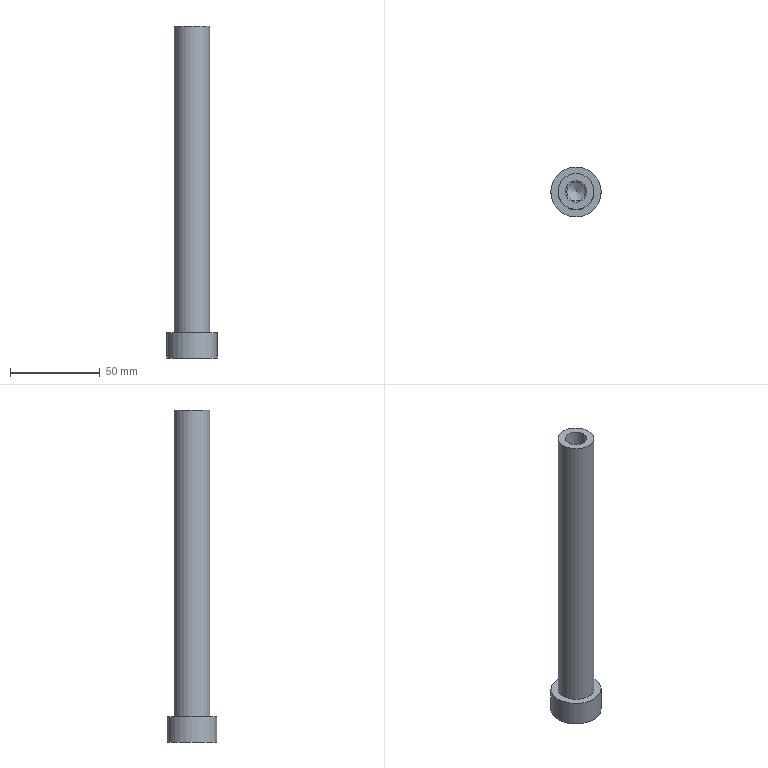Part | STEP file | 1_id670_xmt_txt | 1 solid | 16 faces | box 28 x 28 x 185 mm | volume 57057 mm3 | plane 10 | cylinder 4 | cone 2 | commonest cylinder face diameters 10.2 x1 12 x1 20 x1 28 x1
STEP:
#1=CARTESIAN_POINT('',(-86.,260.,-214.));
#2=VERTEX_POINT('',#1);
#3=CARTESIAN_POINT('',(-100.,260.,-214.));
#4=DIRECTION('',(0.,0.,-1.));
#5=DIRECTION('',(1.,0.,0.));
#6=AXIS2_PLACEMENT_3D('',#3,#4,#5);
#7=CIRCLE('',#6,14.);
#8=EDGE_CURVE('',#2,#2,#7,.T.);
#9=ORIENTED_EDGE('',*,*,#8,.F.);
#10=EDGE_LOOP('',(#9));
#11=FACE_BOUND('',#10,.T.);
#12=CARTESIAN_POINT('',(-86.,260.,-200.));
#13=VERTEX_POINT('',#12);
#14=CARTESIAN_POINT('',(-100.,260.,-200.));
#15=DIRECTION('',(0.,0.,1.));
#16=DIRECTION('',(1.,0.,0.));
#17=AXIS2_PLACEMENT_3D('',#14,#15,#16);
#18=CIRCLE('',#17,14.);
#19=EDGE_CURVE('',#13,#13,#18,.T.);
#20=ORIENTED_EDGE('',*,*,#19,.F.);
#21=EDGE_LOOP('',(#20));
#22=FACE_BOUND('',#21,.T.);
#23=CARTESIAN_POINT('',(-100.,260.,-207.));
#24=DIRECTION('',(0.,0.,1.));
#25=DIRECTION('',(-1.,0.,0.));
#26=AXIS2_PLACEMENT_3D('',#23,#24,#25);
#27=CYLINDRICAL_SURFACE('',#26,14.);
#28=ADVANCED_FACE('',(#11,#22),#27,.T.);
#29=CARTESIAN_POINT('',(-90.,260.,-200.));
#30=VERTEX_POINT('',#29);
#31=CARTESIAN_POINT('',(-100.,260.,-200.));
#32=DIRECTION('',(0.,0.,-1.));
#33=DIRECTION('',(1.,0.,0.));
#34=AXIS2_PLACEMENT_3D('',#31,#32,#33);
#35=CIRCLE('',#34,10.);
#36=EDGE_CURVE('',#30,#30,#35,.T.);
#37=ORIENTED_EDGE('',*,*,#36,.F.);
#38=EDGE_LOOP('',(#37));
#39=FACE_BOUND('',#38,.T.);
#40=CARTESIAN_POINT('',(-90.,260.,-29.));
#41=VERTEX_POINT('',#40);
#42=CARTESIAN_POINT('',(-100.,260.,-29.));
#43=DIRECTION('',(0.,0.,1.));
#44=DIRECTION('',(1.,0.,0.));
#45=AXIS2_PLACEMENT_3D('',#42,#43,#44);
#46=CIRCLE('',#45,10.);
#47=EDGE_CURVE('',#41,#41,#46,.T.);
#48=ORIENTED_EDGE('',*,*,#47,.F.);
#49=EDGE_LOOP('',(#48));
#50=FACE_BOUND('',#49,.T.);
#51=CARTESIAN_POINT('',(-100.,260.,-115.));
#52=DIRECTION('',(0.,0.,1.));
#53=DIRECTION('',(-1.,0.,0.));
#54=AXIS2_PLACEMENT_3D('',#51,#52,#53);
#55=CYLINDRICAL_SURFACE('',#54,10.);
#56=ADVANCED_FACE('',(#39,#50),#55,.T.);
#57=CARTESIAN_POINT('',(-106.,260.,-60.));
#58=VERTEX_POINT('',#57);
#59=CARTESIAN_POINT('',(-100.,260.,-60.));
#60=DIRECTION('',(0.,0.,-1.));
#61=DIRECTION('',(-1.,0.,0.));
#62=AXIS2_PLACEMENT_3D('',#59,#60,#61);
#63=CIRCLE('',#62,6.);
#64=EDGE_CURVE('',#58,#58,#63,.T.);
#65=ORIENTED_EDGE('',*,*,#64,.T.);
#66=EDGE_LOOP('',(#65));
#67=FACE_BOUND('',#66,.T.);
#68=CARTESIAN_POINT('',(-106.,260.,-29.));
#69=VERTEX_POINT('',#68);
#70=CARTESIAN_POINT('',(-100.,260.,-29.));
#71=DIRECTION('',(0.,0.,-1.));
#72=DIRECTION('',(-1.,0.,0.));
#73=AXIS2_PLACEMENT_3D('',#70,#71,#72);
#74=CIRCLE('',#73,6.);
#75=EDGE_CURVE('',#69,#69,#74,.T.);
#76=ORIENTED_EDGE('',*,*,#75,.F.);
#77=EDGE_LOOP('',(#76));
#78=FACE_BOUND('',#77,.T.);
#79=CARTESIAN_POINT('',(-100.,260.,-45.));
#80=DIRECTION('',(0.,0.,-1.));
#81=DIRECTION('',(1.,0.,0.));
#82=AXIS2_PLACEMENT_3D('',#79,#80,#81);
#83=CYLINDRICAL_SURFACE('',#82,6.);
#84=ADVANCED_FACE('',(#67,#78),#83,.F.);
#85=CARTESIAN_POINT('',(-105.1,260.,-60.5));
#86=VERTEX_POINT('',#85);
#87=CARTESIAN_POINT('',(-100.,260.,-60.5));
#88=DIRECTION('',(0.,0.,-1.));
#89=DIRECTION('',(-1.,0.,0.));
#90=AXIS2_PLACEMENT_3D('',#87,#88,#89);
#91=CIRCLE('',#90,5.1);
#92=EDGE_CURVE('',#86,#86,#91,.T.);
#93=ORIENTED_EDGE('',*,*,#92,.T.);
#94=EDGE_LOOP('',(#93));
#95=FACE_BOUND('',#94,.T.);
#96=ORIENTED_EDGE('',*,*,#64,.F.);
#97=EDGE_LOOP('',(#96));
#98=FACE_BOUND('',#97,.T.);
#99=CARTESIAN_POINT('',(-100.,260.,-60.25));
#100=DIRECTION('',(0.,0.,1.));
#101=DIRECTION('',(1.,0.,0.));
#102=AXIS2_PLACEMENT_3D('',#99,#100,#101);
#103=CONICAL_SURFACE('',#102,5.55,60.945);
#104=ADVANCED_FACE('',(#95,#98),#103,.F.);
#105=CARTESIAN_POINT('',(-105.1,260.,-62.));
#106=VERTEX_POINT('',#105);
#107=CARTESIAN_POINT('',(-100.,260.,-62.));
#108=DIRECTION('',(0.,0.,-1.));
#109=DIRECTION('',(-1.,0.,0.));
#110=AXIS2_PLACEMENT_3D('',#107,#108,#109);
#111=CIRCLE('',#110,5.1);
#112=EDGE_CURVE('',#106,#106,#111,.T.);
#113=ORIENTED_EDGE('',*,*,#112,.T.);
#114=EDGE_LOOP('',(#113));
#115=FACE_BOUND('',#114,.T.);
#116=ORIENTED_EDGE('',*,*,#92,.F.);
#117=EDGE_LOOP('',(#116));
#118=FACE_BOUND('',#117,.T.);
#119=CARTESIAN_POINT('',(-100.,260.,-61.25));
#120=DIRECTION('',(0.,0.,-1.));
#121=DIRECTION('',(1.,0.,0.));
#122=AXIS2_PLACEMENT_3D('',#119,#120,#121);
#123=CYLINDRICAL_SURFACE('',#122,5.1);
#124=ADVANCED_FACE('',(#115,#118),#123,.F.);
#125=ORIENTED_EDGE('',*,*,#112,.F.);
#126=EDGE_LOOP('',(#125));
#127=FACE_BOUND('',#126,.T.);
#128=CARTESIAN_POINT('',(-100.,260.,-64.944));
#129=VERTEX_POINT('',#128);
#130=VERTEX_LOOP('',#129);
#131=FACE_BOUND('',#130,.T.);
#132=CARTESIAN_POINT('',(-100.,260.,-63.472));
#133=DIRECTION('',(0.,0.,1.));
#134=DIRECTION('',(1.,0.,0.));
#135=AXIS2_PLACEMENT_3D('',#132,#133,#134);
#136=CONICAL_SURFACE('',#135,2.55,60.);
#137=ADVANCED_FACE('',(#127,#131),#136,.F.);
#138=CARTESIAN_POINT('',(-104.041,267.,-205.));
#139=VERTEX_POINT('',#138);
#140=CARTESIAN_POINT('',(-95.959,267.,-205.));
#141=VERTEX_POINT('',#140);
#142=CARTESIAN_POINT('',(-104.041,267.,-205.));
#143=DIRECTION('',(1.,0.,0.));
#144=VECTOR('',#143,1.);
#145=LINE('',#142,#144);
#146=EDGE_CURVE('',#139,#141,#145,.T.);
#147=ORIENTED_EDGE('',*,*,#146,.F.);
#148=CARTESIAN_POINT('',(-104.041,267.,-214.));
#149=VERTEX_POINT('',#148);
#150=CARTESIAN_POINT('',(-104.041,267.,-214.));
#151=DIRECTION('',(0.,0.,1.));
#152=VECTOR('',#151,1.);
#153=LINE('',#150,#152);
#154=EDGE_CURVE('',#149,#139,#153,.T.);
#155=ORIENTED_EDGE('',*,*,#154,.F.);
#156=CARTESIAN_POINT('',(-95.959,267.,-214.));
#157=VERTEX_POINT('',#156);
#158=CARTESIAN_POINT('',(-100.,267.,-214.));
#159=DIRECTION('',(-1.,0.,0.));
#160=VECTOR('',#159,1.);
#161=LINE('',#158,#160);
#162=EDGE_CURVE('',#157,#149,#161,.T.);
#163=ORIENTED_EDGE('',*,*,#162,.F.);
#164=CARTESIAN_POINT('',(-95.959,267.,-214.));
#165=DIRECTION('',(0.,0.,1.));
#166=VECTOR('',#165,1.);
#167=LINE('',#164,#166);
#168=EDGE_CURVE('',#157,#141,#167,.T.);
#169=ORIENTED_EDGE('',*,*,#168,.T.);
#170=EDGE_LOOP('',(#147,#155,#163,#169));
#171=FACE_OUTER_BOUND('',#170,.T.);
#172=CARTESIAN_POINT('',(-100.,267.,-214.));
#173=DIRECTION('',(0.,1.,0.));
#174=DIRECTION('',(1.,0.,0.));
#175=AXIS2_PLACEMENT_3D('',#172,#173,#174);
#176=PLANE('',#175);
#177=ADVANCED_FACE('',(#171),#176,.F.);
#178=CARTESIAN_POINT('',(-91.917,260.,-205.));
#179=VERTEX_POINT('',#178);
#180=CARTESIAN_POINT('',(-95.959,267.,-205.));
#181=DIRECTION('',(0.5,-0.866,0.));
#182=VECTOR('',#181,1.);
#183=LINE('',#180,#182);
#184=EDGE_CURVE('',#141,#179,#183,.T.);
#185=ORIENTED_EDGE('',*,*,#184,.F.);
#186=ORIENTED_EDGE('',*,*,#168,.F.);
#187=CARTESIAN_POINT('',(-91.917,260.,-214.));
#188=VERTEX_POINT('',#187);
#189=CARTESIAN_POINT('',(-93.938,263.5,-214.));
#190=DIRECTION('',(-0.5,0.866,0.));
#191=VECTOR('',#190,1.);
#192=LINE('',#189,#191);
#193=EDGE_CURVE('',#188,#157,#192,.T.);
#194=ORIENTED_EDGE('',*,*,#193,.F.);
#195=CARTESIAN_POINT('',(-91.917,260.,-214.));
#196=DIRECTION('',(0.,0.,1.));
#197=VECTOR('',#196,1.);
#198=LINE('',#195,#197);
#199=EDGE_CURVE('',#188,#179,#198,.T.);
#200=ORIENTED_EDGE('',*,*,#199,.T.);
#201=EDGE_LOOP('',(#185,#186,#194,#200));
#202=FACE_OUTER_BOUND('',#201,.T.);
#203=CARTESIAN_POINT('',(-93.938,263.5,-214.));
#204=DIRECTION('',(0.866,0.5,0.));
#205=DIRECTION('',(0.5,-0.866,0.));
#206=AXIS2_PLACEMENT_3D('',#203,#204,#205);
#207=PLANE('',#206);
#208=ADVANCED_FACE('',(#202),#207,.F.);
#209=CARTESIAN_POINT('',(-95.959,253.,-205.));
#210=VERTEX_POINT('',#209);
#211=CARTESIAN_POINT('',(-91.917,260.,-205.));
#212=DIRECTION('',(-0.5,-0.866,0.));
#213=VECTOR('',#212,1.);
#214=LINE('',#211,#213);
#215=EDGE_CURVE('',#179,#210,#214,.T.);
#216=ORIENTED_EDGE('',*,*,#215,.F.);
#217=ORIENTED_EDGE('',*,*,#199,.F.);
#218=CARTESIAN_POINT('',(-95.959,253.,-214.));
#219=VERTEX_POINT('',#218);
#220=CARTESIAN_POINT('',(-93.938,256.5,-214.));
#221=DIRECTION('',(0.5,0.866,0.));
#222=VECTOR('',#221,1.);
#223=LINE('',#220,#222);
#224=EDGE_CURVE('',#219,#188,#223,.T.);
#225=ORIENTED_EDGE('',*,*,#224,.F.);
#226=CARTESIAN_POINT('',(-95.959,253.,-214.));
#227=DIRECTION('',(0.,0.,1.));
#228=VECTOR('',#227,1.);
#229=LINE('',#226,#228);
#230=EDGE_CURVE('',#219,#210,#229,.T.);
#231=ORIENTED_EDGE('',*,*,#230,.T.);
#232=EDGE_LOOP('',(#216,#217,#225,#231));
#233=FACE_OUTER_BOUND('',#232,.T.);
#234=CARTESIAN_POINT('',(-93.938,256.5,-214.));
#235=DIRECTION('',(0.866,-0.5,0.));
#236=DIRECTION('',(-0.5,-0.866,0.));
#237=AXIS2_PLACEMENT_3D('',#234,#235,#236);
#238=PLANE('',#237);
#239=ADVANCED_FACE('',(#233),#238,.F.);
#240=CARTESIAN_POINT('',(-104.041,253.,-205.));
#241=VERTEX_POINT('',#240);
#242=CARTESIAN_POINT('',(-95.959,253.,-205.));
#243=DIRECTION('',(-1.,0.,0.));
#244=VECTOR('',#243,1.);
#245=LINE('',#242,#244);
#246=EDGE_CURVE('',#210,#241,#245,.T.);
#247=ORIENTED_EDGE('',*,*,#246,.F.);
#248=ORIENTED_EDGE('',*,*,#230,.F.);
#249=CARTESIAN_POINT('',(-104.041,253.,-214.));
#250=VERTEX_POINT('',#249);
#251=CARTESIAN_POINT('',(-100.,253.,-214.));
#252=DIRECTION('',(1.,0.,0.));
#253=VECTOR('',#252,1.);
#254=LINE('',#251,#253);
#255=EDGE_CURVE('',#250,#219,#254,.T.);
#256=ORIENTED_EDGE('',*,*,#255,.F.);
#257=CARTESIAN_POINT('',(-104.041,253.,-214.));
#258=DIRECTION('',(0.,0.,1.));
#259=VECTOR('',#258,1.);
#260=LINE('',#257,#259);
#261=EDGE_CURVE('',#250,#241,#260,.T.);
#262=ORIENTED_EDGE('',*,*,#261,.T.);
#263=EDGE_LOOP('',(#247,#248,#256,#262));
#264=FACE_OUTER_BOUND('',#263,.T.);
#265=CARTESIAN_POINT('',(-100.,253.,-214.));
#266=DIRECTION('',(0.,-1.,0.));
#267=DIRECTION('',(-1.,0.,0.));
#268=AXIS2_PLACEMENT_3D('',#265,#266,#267);
#269=PLANE('',#268);
#270=ADVANCED_FACE('',(#264),#269,.F.);
#271=CARTESIAN_POINT('',(-108.083,260.,-205.));
#272=VERTEX_POINT('',#271);
#273=CARTESIAN_POINT('',(-104.041,253.,-205.));
#274=DIRECTION('',(-0.5,0.866,0.));
#275=VECTOR('',#274,1.);
#276=LINE('',#273,#275);
#277=EDGE_CURVE('',#241,#272,#276,.T.);
#278=ORIENTED_EDGE('',*,*,#277,.F.);
#279=ORIENTED_EDGE('',*,*,#261,.F.);
#280=CARTESIAN_POINT('',(-108.083,260.,-214.));
#281=VERTEX_POINT('',#280);
#282=CARTESIAN_POINT('',(-106.062,256.5,-214.));
#283=DIRECTION('',(0.5,-0.866,0.));
#284=VECTOR('',#283,1.);
#285=LINE('',#282,#284);
#286=EDGE_CURVE('',#281,#250,#285,.T.);
#287=ORIENTED_EDGE('',*,*,#286,.F.);
#288=CARTESIAN_POINT('',(-108.083,260.,-214.));
#289=DIRECTION('',(0.,0.,1.));
#290=VECTOR('',#289,1.);
#291=LINE('',#288,#290);
#292=EDGE_CURVE('',#281,#272,#291,.T.);
#293=ORIENTED_EDGE('',*,*,#292,.T.);
#294=EDGE_LOOP('',(#278,#279,#287,#293));
#295=FACE_OUTER_BOUND('',#294,.T.);
#296=CARTESIAN_POINT('',(-106.062,256.5,-214.));
#297=DIRECTION('',(-0.866,-0.5,0.));
#298=DIRECTION('',(-0.5,0.866,0.));
#299=AXIS2_PLACEMENT_3D('',#296,#297,#298);
#300=PLANE('',#299);
#301=ADVANCED_FACE('',(#295),#300,.F.);
#302=CARTESIAN_POINT('',(-108.083,260.,-205.));
#303=DIRECTION('',(0.5,0.866,0.));
#304=VECTOR('',#303,1.);
#305=LINE('',#302,#304);
#306=EDGE_CURVE('',#272,#139,#305,.T.);
#307=ORIENTED_EDGE('',*,*,#306,.F.);
#308=ORIENTED_EDGE('',*,*,#292,.F.);
#309=CARTESIAN_POINT('',(-106.062,263.5,-214.));
#310=DIRECTION('',(-0.5,-0.866,0.));
#311=VECTOR('',#310,1.);
#312=LINE('',#309,#311);
#313=EDGE_CURVE('',#149,#281,#312,.T.);
#314=ORIENTED_EDGE('',*,*,#313,.F.);
#315=ORIENTED_EDGE('',*,*,#154,.T.);
#316=EDGE_LOOP('',(#307,#308,#314,#315));
#317=FACE_OUTER_BOUND('',#316,.T.);
#318=CARTESIAN_POINT('',(-106.062,263.5,-214.));
#319=DIRECTION('',(-0.866,0.5,0.));
#320=DIRECTION('',(0.5,0.866,0.));
#321=AXIS2_PLACEMENT_3D('',#318,#319,#320);
#322=PLANE('',#321);
#323=ADVANCED_FACE('',(#317),#322,.F.);
#324=ORIENTED_EDGE('',*,*,#146,.T.);
#325=ORIENTED_EDGE('',*,*,#184,.T.);
#326=ORIENTED_EDGE('',*,*,#215,.T.);
#327=ORIENTED_EDGE('',*,*,#246,.T.);
#328=ORIENTED_EDGE('',*,*,#277,.T.);
#329=ORIENTED_EDGE('',*,*,#306,.T.);
#330=EDGE_LOOP('',(#324,#325,#326,#327,#328,#329));
#331=FACE_OUTER_BOUND('',#330,.T.);
#332=CARTESIAN_POINT('',(-100.,260.,-205.));
#333=DIRECTION('',(0.,0.,1.));
#334=DIRECTION('',(-1.,0.,0.));
#335=AXIS2_PLACEMENT_3D('',#332,#333,#334);
#336=PLANE('',#335);
#337=ADVANCED_FACE('',(#331),#336,.F.);
#338=ORIENTED_EDGE('',*,*,#75,.T.);
#339=EDGE_LOOP('',(#338));
#340=FACE_BOUND('',#339,.T.);
#341=ORIENTED_EDGE('',*,*,#47,.T.);
#342=EDGE_LOOP('',(#341));
#343=FACE_BOUND('',#342,.T.);
#344=CARTESIAN_POINT('',(-100.,260.,-29.));
#345=DIRECTION('',(0.,0.,1.));
#346=DIRECTION('',(-1.,0.,0.));
#347=AXIS2_PLACEMENT_3D('',#344,#345,#346);
#348=PLANE('',#347);
#349=ADVANCED_FACE('',(#340,#343),#348,.T.);
#350=ORIENTED_EDGE('',*,*,#162,.T.);
#351=ORIENTED_EDGE('',*,*,#313,.T.);
#352=ORIENTED_EDGE('',*,*,#286,.T.);
#353=ORIENTED_EDGE('',*,*,#255,.T.);
#354=ORIENTED_EDGE('',*,*,#224,.T.);
#355=ORIENTED_EDGE('',*,*,#193,.T.);
#356=EDGE_LOOP('',(#350,#351,#352,#353,#354,#355));
#357=FACE_BOUND('',#356,.T.);
#358=ORIENTED_EDGE('',*,*,#8,.T.);
#359=EDGE_LOOP('',(#358));
#360=FACE_BOUND('',#359,.T.);
#361=CARTESIAN_POINT('',(-100.,260.,-214.));
#362=DIRECTION('',(0.,0.,-1.));
#363=DIRECTION('',(1.,0.,0.));
#364=AXIS2_PLACEMENT_3D('',#361,#362,#363);
#365=PLANE('',#364);
#366=ADVANCED_FACE('',(#357,#360),#365,.T.);
#367=ORIENTED_EDGE('',*,*,#36,.T.);
#368=EDGE_LOOP('',(#367));
#369=FACE_BOUND('',#368,.T.);
#370=ORIENTED_EDGE('',*,*,#19,.T.);
#371=EDGE_LOOP('',(#370));
#372=FACE_BOUND('',#371,.T.);
#373=CARTESIAN_POINT('',(-100.,260.,-200.));
#374=DIRECTION('',(0.,0.,1.));
#375=DIRECTION('',(-1.,0.,0.));
#376=AXIS2_PLACEMENT_3D('',#373,#374,#375);
#377=PLANE('',#376);
#378=ADVANCED_FACE('',(#369,#372),#377,.T.);
#379=CLOSED_SHELL('',(#28,#56,#84,#104,#124,#137,#177,#208,#239,#270,#301,#323,#337,#349,#366,#378));
#380=MANIFOLD_SOLID_BREP('',#379);
#381=(LENGTH_UNIT()NAMED_UNIT(*)SI_UNIT(.MILLI.,.METRE.));
#382=UNCERTAINTY_MEASURE_WITH_UNIT(LENGTH_MEASURE(0.00002),#381,'','');
#383=(NAMED_UNIT(*)PLANE_ANGLE_UNIT()SI_UNIT($,.RADIAN.));
#384=PLANE_ANGLE_MEASURE_WITH_UNIT(PLANE_ANGLE_MEASURE(0.01745),#383);
#385=DIMENSIONAL_EXPONENTS(0.,0.,0.,0.,0.,0.,0.);
#386=(CONVERSION_BASED_UNIT('DEGREE',#384)NAMED_UNIT(#385)PLANE_ANGLE_UNIT());
#387=(NAMED_UNIT(*)SI_UNIT($,.STERADIAN.)SOLID_ANGLE_UNIT());
#388=(GEOMETRIC_REPRESENTATION_CONTEXT(3)GLOBAL_UNCERTAINTY_ASSIGNED_CONTEXT((#382))GLOBAL_UNIT_ASSIGNED_CONTEXT((#381,#386,#387))REPRESENTATION_CONTEXT('',''));
#389=ADVANCED_BREP_SHAPE_REPRESENTATION('',(#380),#388);